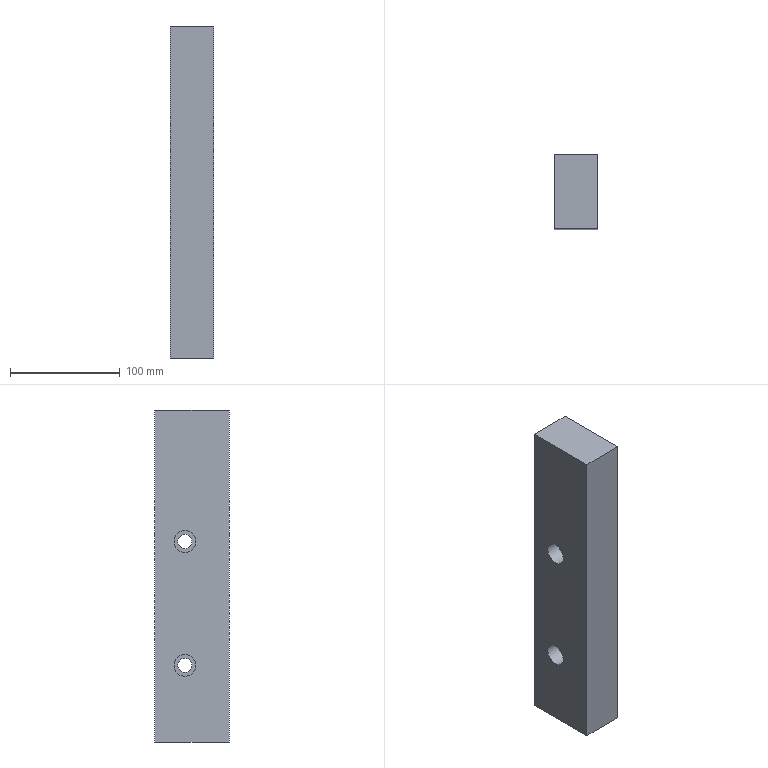Part | NX | features solid 2 | 1 solid | 12 faces | box 40 x 67.998 x 303 mm | volume 806258 mm3 | plane 8 | cylinder 4 | commonest cylinder face diameters 13 x2 20 x2
STEP:
#1=CARTESIAN_POINT('',(300.,-447.002,480.));
#2=VERTEX_POINT('',#1);
#3=CARTESIAN_POINT('',(300.,-515.,480.));
#4=VERTEX_POINT('',#3);
#5=CARTESIAN_POINT('',(300.,373.333,480.));
#6=DIRECTION('',(0.,-1.,0.));
#7=VECTOR('',#6,1000.);
#8=LINE('',#5,#7);
#9=EDGE_CURVE('',#2,#4,#8,.T.);
#10=ORIENTED_EDGE('',*,*,#9,.F.);
#11=CARTESIAN_POINT('',(260.,-447.002,480.));
#12=VERTEX_POINT('',#11);
#13=CARTESIAN_POINT('',(236.145,-447.002,480.));
#14=DIRECTION('',(-1.,0.,0.));
#15=VECTOR('',#14,1000.);
#16=LINE('',#13,#15);
#17=EDGE_CURVE('',#12,#2,#16,.F.);
#18=ORIENTED_EDGE('',*,*,#17,.F.);
#19=CARTESIAN_POINT('',(260.,-515.,480.));
#20=VERTEX_POINT('',#19);
#21=CARTESIAN_POINT('',(260.,373.333,480.));
#22=DIRECTION('',(0.,-1.,0.));
#23=VECTOR('',#22,1000.);
#24=LINE('',#21,#23);
#25=EDGE_CURVE('',#12,#20,#24,.T.);
#26=ORIENTED_EDGE('',*,*,#25,.T.);
#27=CARTESIAN_POINT('',(236.145,-515.,480.));
#28=DIRECTION('',(1.,0.,0.));
#29=VECTOR('',#28,1000.);
#30=LINE('',#27,#29);
#31=EDGE_CURVE('',#20,#4,#30,.T.);
#32=ORIENTED_EDGE('',*,*,#31,.T.);
#33=EDGE_LOOP('',(#10,#18,#26,#32));
#34=FACE_BOUND('',#33,.T.);
#35=CARTESIAN_POINT('',(236.145,373.333,480.));
#36=DIRECTION('',(0.,0.,1.));
#37=DIRECTION('',(1.,0.,0.));
#38=AXIS2_PLACEMENT_3D('',#35,#36,#37);
#39=PLANE('',#38);
#40=ADVANCED_FACE('',(#34),#39,.T.);
#41=CARTESIAN_POINT('',(300.,-447.002,177.));
#42=VERTEX_POINT('',#41);
#43=CARTESIAN_POINT('',(300.,-447.002,482.));
#44=DIRECTION('',(0.,0.,1.));
#45=VECTOR('',#44,1000.);
#46=LINE('',#43,#45);
#47=EDGE_CURVE('',#2,#42,#46,.F.);
#48=ORIENTED_EDGE('',*,*,#47,.T.);
#49=CARTESIAN_POINT('',(260.,-447.002,177.));
#50=VERTEX_POINT('',#49);
#51=CARTESIAN_POINT('',(296.145,-447.002,177.));
#52=DIRECTION('',(-1.,0.,0.));
#53=VECTOR('',#52,1000.);
#54=LINE('',#51,#53);
#55=EDGE_CURVE('',#50,#42,#54,.F.);
#56=ORIENTED_EDGE('',*,*,#55,.F.);
#57=CARTESIAN_POINT('',(260.,-447.002,482.));
#58=DIRECTION('',(0.,0.,1.));
#59=VECTOR('',#58,1000.);
#60=LINE('',#57,#59);
#61=EDGE_CURVE('',#12,#50,#60,.F.);
#62=ORIENTED_EDGE('',*,*,#61,.F.);
#63=ORIENTED_EDGE('',*,*,#17,.T.);
#64=EDGE_LOOP('',(#48,#56,#62,#63));
#65=FACE_BOUND('',#64,.T.);
#66=CARTESIAN_POINT('',(296.145,-447.002,482.));
#67=DIRECTION('',(0.,1.,0.));
#68=DIRECTION('',(0.,0.,1.));
#69=AXIS2_PLACEMENT_3D('',#66,#67,#68);
#70=PLANE('',#69);
#71=ADVANCED_FACE('',(#65),#70,.T.);
#72=CARTESIAN_POINT('',(300.,-515.,177.));
#73=VERTEX_POINT('',#72);
#74=CARTESIAN_POINT('',(300.,-517.002,177.));
#75=DIRECTION('',(0.,1.,0.));
#76=VECTOR('',#75,1000.);
#77=LINE('',#74,#76);
#78=EDGE_CURVE('',#73,#42,#77,.T.);
#79=ORIENTED_EDGE('',*,*,#78,.F.);
#80=CARTESIAN_POINT('',(260.,-515.,177.));
#81=VERTEX_POINT('',#80);
#82=CARTESIAN_POINT('',(236.145,-515.,177.));
#83=DIRECTION('',(1.,0.,0.));
#84=VECTOR('',#83,1000.);
#85=LINE('',#82,#84);
#86=EDGE_CURVE('',#81,#73,#85,.T.);
#87=ORIENTED_EDGE('',*,*,#86,.F.);
#88=CARTESIAN_POINT('',(260.,-517.002,177.));
#89=DIRECTION('',(0.,1.,0.));
#90=VECTOR('',#89,1000.);
#91=LINE('',#88,#90);
#92=EDGE_CURVE('',#81,#50,#91,.T.);
#93=ORIENTED_EDGE('',*,*,#92,.T.);
#94=ORIENTED_EDGE('',*,*,#55,.T.);
#95=EDGE_LOOP('',(#79,#87,#93,#94));
#96=FACE_BOUND('',#95,.T.);
#97=CARTESIAN_POINT('',(236.145,-517.002,177.));
#98=DIRECTION('',(0.,0.,-1.));
#99=DIRECTION('',(-1.,0.,0.));
#100=AXIS2_PLACEMENT_3D('',#97,#98,#99);
#101=PLANE('',#100);
#102=ADVANCED_FACE('',(#96),#101,.T.);
#103=CARTESIAN_POINT('',(300.,-515.,482.));
#104=DIRECTION('',(0.,0.,-1.));
#105=VECTOR('',#104,1000.);
#106=LINE('',#103,#105);
#107=EDGE_CURVE('',#4,#73,#106,.T.);
#108=ORIENTED_EDGE('',*,*,#107,.F.);
#109=ORIENTED_EDGE('',*,*,#31,.F.);
#110=CARTESIAN_POINT('',(260.,-515.,482.));
#111=DIRECTION('',(0.,0.,-1.));
#112=VECTOR('',#111,1000.);
#113=LINE('',#110,#112);
#114=EDGE_CURVE('',#20,#81,#113,.T.);
#115=ORIENTED_EDGE('',*,*,#114,.T.);
#116=ORIENTED_EDGE('',*,*,#86,.T.);
#117=EDGE_LOOP('',(#108,#109,#115,#116));
#118=FACE_BOUND('',#117,.T.);
#119=CARTESIAN_POINT('',(236.145,-515.,482.));
#120=DIRECTION('',(0.,-1.,0.));
#121=DIRECTION('',(0.,0.,-1.));
#122=AXIS2_PLACEMENT_3D('',#119,#120,#121);
#123=PLANE('',#122);
#124=ADVANCED_FACE('',(#118),#123,.T.);
#125=CARTESIAN_POINT('',(260.,-474.502,370.));
#126=VERTEX_POINT('',#125);
#127=CARTESIAN_POINT('',(260.,-474.502,360.));
#128=DIRECTION('',(-1.,0.,0.));
#129=DIRECTION('',(0.,0.,1.));
#130=AXIS2_PLACEMENT_3D('',#127,#128,#129);
#131=CIRCLE('',#130,10.);
#132=EDGE_CURVE('',#126,#126,#131,.T.);
#133=ORIENTED_EDGE('',*,*,#132,.F.);
#134=EDGE_LOOP('',(#133));
#135=FACE_BOUND('',#134,.T.);
#136=CARTESIAN_POINT('',(260.,-474.502,257.));
#137=VERTEX_POINT('',#136);
#138=CARTESIAN_POINT('',(260.,-474.502,247.));
#139=DIRECTION('',(-1.,0.,0.));
#140=DIRECTION('',(0.,0.,1.));
#141=AXIS2_PLACEMENT_3D('',#138,#139,#140);
#142=CIRCLE('',#141,10.);
#143=EDGE_CURVE('',#137,#137,#142,.T.);
#144=ORIENTED_EDGE('',*,*,#143,.F.);
#145=EDGE_LOOP('',(#144));
#146=FACE_BOUND('',#145,.T.);
#147=ORIENTED_EDGE('',*,*,#25,.F.);
#148=ORIENTED_EDGE('',*,*,#61,.T.);
#149=ORIENTED_EDGE('',*,*,#92,.F.);
#150=ORIENTED_EDGE('',*,*,#114,.F.);
#151=EDGE_LOOP('',(#147,#148,#149,#150));
#152=FACE_BOUND('',#151,.T.);
#153=CARTESIAN_POINT('',(260.,-517.002,482.));
#154=DIRECTION('',(-1.,0.,0.));
#155=DIRECTION('',(0.,0.,-1.));
#156=AXIS2_PLACEMENT_3D('',#153,#154,#155);
#157=PLANE('',#156);
#158=ADVANCED_FACE('',(#135,#146,#152),#157,.T.);
#159=CARTESIAN_POINT('',(300.,-474.502,366.5));
#160=VERTEX_POINT('',#159);
#161=CARTESIAN_POINT('',(300.,-474.502,360.));
#162=DIRECTION('',(-1.,0.,0.));
#163=DIRECTION('',(0.,0.,1.));
#164=AXIS2_PLACEMENT_3D('',#161,#162,#163);
#165=CIRCLE('',#164,6.5);
#166=EDGE_CURVE('',#160,#160,#165,.T.);
#167=ORIENTED_EDGE('',*,*,#166,.T.);
#168=EDGE_LOOP('',(#167));
#169=FACE_BOUND('',#168,.T.);
#170=CARTESIAN_POINT('',(300.,-474.502,253.5));
#171=VERTEX_POINT('',#170);
#172=CARTESIAN_POINT('',(300.,-474.502,247.));
#173=DIRECTION('',(-1.,0.,0.));
#174=DIRECTION('',(0.,0.,1.));
#175=AXIS2_PLACEMENT_3D('',#172,#173,#174);
#176=CIRCLE('',#175,6.5);
#177=EDGE_CURVE('',#171,#171,#176,.T.);
#178=ORIENTED_EDGE('',*,*,#177,.T.);
#179=EDGE_LOOP('',(#178));
#180=FACE_BOUND('',#179,.T.);
#181=ORIENTED_EDGE('',*,*,#9,.T.);
#182=ORIENTED_EDGE('',*,*,#107,.T.);
#183=ORIENTED_EDGE('',*,*,#78,.T.);
#184=ORIENTED_EDGE('',*,*,#47,.F.);
#185=EDGE_LOOP('',(#181,#182,#183,#184));
#186=FACE_BOUND('',#185,.T.);
#187=CARTESIAN_POINT('',(300.,-517.002,482.));
#188=DIRECTION('',(-1.,0.,0.));
#189=DIRECTION('',(0.,0.,-1.));
#190=AXIS2_PLACEMENT_3D('',#187,#188,#189);
#191=PLANE('',#190);
#192=ADVANCED_FACE('',(#169,#180,#186),#191,.F.);
#193=CARTESIAN_POINT('',(280.,-474.502,240.5));
#194=VERTEX_POINT('',#193);
#195=CARTESIAN_POINT('',(280.,-474.502,247.));
#196=DIRECTION('',(1.,0.,0.));
#197=DIRECTION('',(0.,0.,-1.));
#198=AXIS2_PLACEMENT_3D('',#195,#196,#197);
#199=CIRCLE('',#198,6.5);
#200=EDGE_CURVE('',#194,#194,#199,.F.);
#201=ORIENTED_EDGE('',*,*,#200,.T.);
#202=EDGE_LOOP('',(#201));
#203=FACE_BOUND('',#202,.T.);
#204=ORIENTED_EDGE('',*,*,#177,.F.);
#205=EDGE_LOOP('',(#204));
#206=FACE_BOUND('',#205,.T.);
#207=CARTESIAN_POINT('',(320.,-474.502,247.));
#208=DIRECTION('',(-1.,0.,0.));
#209=DIRECTION('',(0.,0.,1.));
#210=AXIS2_PLACEMENT_3D('',#207,#208,#209);
#211=CYLINDRICAL_SURFACE('',#210,6.5);
#212=ADVANCED_FACE('',(#203,#206),#211,.F.);
#213=ORIENTED_EDGE('',*,*,#200,.F.);
#214=EDGE_LOOP('',(#213));
#215=FACE_BOUND('',#214,.T.);
#216=CARTESIAN_POINT('',(280.,-474.502,257.));
#217=VERTEX_POINT('',#216);
#218=CARTESIAN_POINT('',(280.,-474.502,247.));
#219=DIRECTION('',(-1.,0.,0.));
#220=DIRECTION('',(0.,0.,1.));
#221=AXIS2_PLACEMENT_3D('',#218,#219,#220);
#222=CIRCLE('',#221,10.);
#223=EDGE_CURVE('',#217,#217,#222,.T.);
#224=ORIENTED_EDGE('',*,*,#223,.T.);
#225=EDGE_LOOP('',(#224));
#226=FACE_BOUND('',#225,.T.);
#227=CARTESIAN_POINT('',(280.,-474.502,247.));
#228=DIRECTION('',(1.,0.,0.));
#229=DIRECTION('',(0.,0.,-1.));
#230=AXIS2_PLACEMENT_3D('',#227,#228,#229);
#231=PLANE('',#230);
#232=ADVANCED_FACE('',(#215,#226),#231,.F.);
#233=ORIENTED_EDGE('',*,*,#143,.T.);
#234=EDGE_LOOP('',(#233));
#235=FACE_BOUND('',#234,.T.);
#236=ORIENTED_EDGE('',*,*,#223,.F.);
#237=EDGE_LOOP('',(#236));
#238=FACE_BOUND('',#237,.T.);
#239=CARTESIAN_POINT('',(280.,-474.502,247.));
#240=DIRECTION('',(-1.,0.,0.));
#241=DIRECTION('',(0.,0.,1.));
#242=AXIS2_PLACEMENT_3D('',#239,#240,#241);
#243=CYLINDRICAL_SURFACE('',#242,10.);
#244=ADVANCED_FACE('',(#235,#238),#243,.F.);
#245=CARTESIAN_POINT('',(280.,-474.502,353.5));
#246=VERTEX_POINT('',#245);
#247=CARTESIAN_POINT('',(280.,-474.502,360.));
#248=DIRECTION('',(1.,0.,0.));
#249=DIRECTION('',(0.,0.,-1.));
#250=AXIS2_PLACEMENT_3D('',#247,#248,#249);
#251=CIRCLE('',#250,6.5);
#252=EDGE_CURVE('',#246,#246,#251,.F.);
#253=ORIENTED_EDGE('',*,*,#252,.T.);
#254=EDGE_LOOP('',(#253));
#255=FACE_BOUND('',#254,.T.);
#256=ORIENTED_EDGE('',*,*,#166,.F.);
#257=EDGE_LOOP('',(#256));
#258=FACE_BOUND('',#257,.T.);
#259=CARTESIAN_POINT('',(320.,-474.502,360.));
#260=DIRECTION('',(-1.,0.,0.));
#261=DIRECTION('',(0.,0.,1.));
#262=AXIS2_PLACEMENT_3D('',#259,#260,#261);
#263=CYLINDRICAL_SURFACE('',#262,6.5);
#264=ADVANCED_FACE('',(#255,#258),#263,.F.);
#265=ORIENTED_EDGE('',*,*,#252,.F.);
#266=EDGE_LOOP('',(#265));
#267=FACE_BOUND('',#266,.T.);
#268=CARTESIAN_POINT('',(280.,-474.502,370.));
#269=VERTEX_POINT('',#268);
#270=CARTESIAN_POINT('',(280.,-474.502,360.));
#271=DIRECTION('',(-1.,0.,0.));
#272=DIRECTION('',(0.,0.,1.));
#273=AXIS2_PLACEMENT_3D('',#270,#271,#272);
#274=CIRCLE('',#273,10.);
#275=EDGE_CURVE('',#269,#269,#274,.T.);
#276=ORIENTED_EDGE('',*,*,#275,.T.);
#277=EDGE_LOOP('',(#276));
#278=FACE_BOUND('',#277,.T.);
#279=CARTESIAN_POINT('',(280.,-474.502,360.));
#280=DIRECTION('',(1.,0.,0.));
#281=DIRECTION('',(0.,0.,-1.));
#282=AXIS2_PLACEMENT_3D('',#279,#280,#281);
#283=PLANE('',#282);
#284=ADVANCED_FACE('',(#267,#278),#283,.F.);
#285=ORIENTED_EDGE('',*,*,#132,.T.);
#286=EDGE_LOOP('',(#285));
#287=FACE_BOUND('',#286,.T.);
#288=ORIENTED_EDGE('',*,*,#275,.F.);
#289=EDGE_LOOP('',(#288));
#290=FACE_BOUND('',#289,.T.);
#291=CARTESIAN_POINT('',(280.,-474.502,360.));
#292=DIRECTION('',(-1.,0.,0.));
#293=DIRECTION('',(0.,0.,1.));
#294=AXIS2_PLACEMENT_3D('',#291,#292,#293);
#295=CYLINDRICAL_SURFACE('',#294,10.);
#296=ADVANCED_FACE('',(#287,#290),#295,.F.);
#297=CLOSED_SHELL('',(#40,#71,#102,#124,#158,#192,#212,#232,#244,#264,#284,#296));
#298=MANIFOLD_SOLID_BREP('',#297);
#299=(LENGTH_UNIT()NAMED_UNIT(*)SI_UNIT(.MILLI.,.METRE.));
#300=UNCERTAINTY_MEASURE_WITH_UNIT(LENGTH_MEASURE(0.00001),#299,'','');
#301=(NAMED_UNIT(*)PLANE_ANGLE_UNIT()SI_UNIT($,.RADIAN.));
#302=(NAMED_UNIT(*)SI_UNIT($,.STERADIAN.)SOLID_ANGLE_UNIT());
#303=(GEOMETRIC_REPRESENTATION_CONTEXT(3)GLOBAL_UNCERTAINTY_ASSIGNED_CONTEXT((#300))GLOBAL_UNIT_ASSIGNED_CONTEXT((#299,#301,#302))REPRESENTATION_CONTEXT('',''));
#304=ADVANCED_BREP_SHAPE_REPRESENTATION('',(#298),#303);